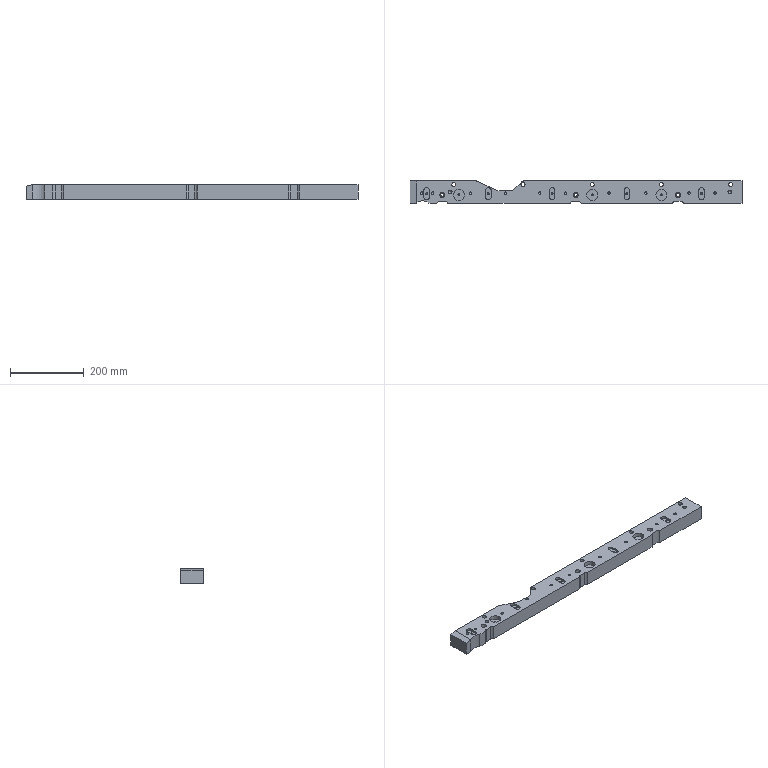Part | NX | features 22 2 | 1 solid | 129 faces | box 902 x 60 x 40 mm | volume 1950233 mm3 | cylinder 64 | plane 45 | cone 20 | commonest cylinder face diameters 6.8 x10 15 x10 14 x9 5.2 x8 6 x6 11 x5